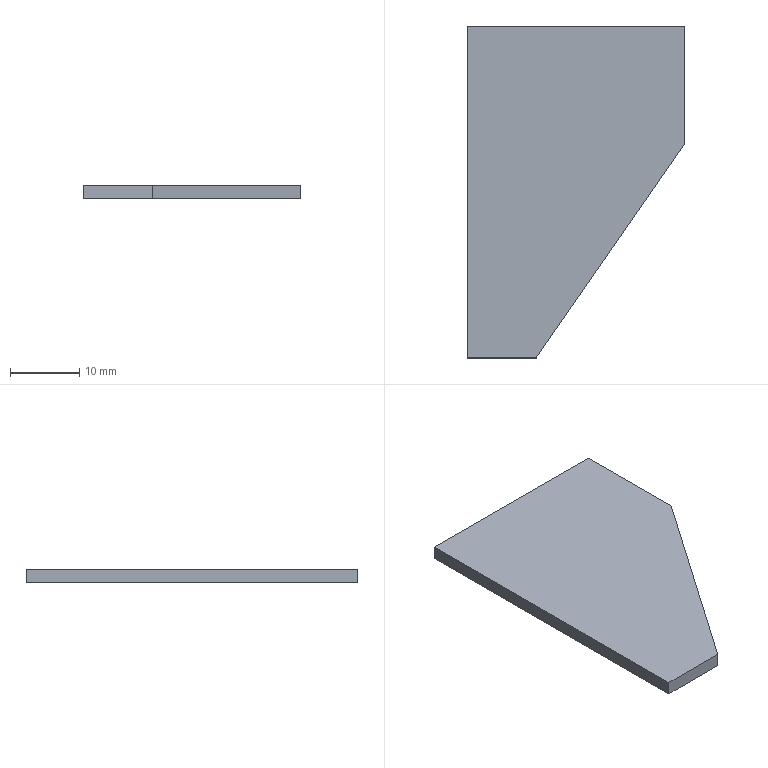Part | 1 solid | 7 faces | box 31.5 x 48 x 2 mm | volume 2357 mm3 | plane 7
STEP:
#1=CARTESIAN_POINT('',(0.,0.,0.));
#2=VERTEX_POINT('',#1);
#3=CARTESIAN_POINT('',(0.,-48.,0.));
#4=VERTEX_POINT('',#3);
#5=CARTESIAN_POINT('',(0.,-48.,0.));
#6=DIRECTION('',(0.,-1.,0.));
#7=VECTOR('',#6,1000.);
#8=LINE('',#5,#7);
#9=EDGE_CURVE('',#2,#4,#8,.T.);
#10=ORIENTED_EDGE('',*,*,#9,.T.);
#11=CARTESIAN_POINT('',(0.,-48.,2.));
#12=VERTEX_POINT('',#11);
#13=CARTESIAN_POINT('',(0.,-48.,2.));
#14=DIRECTION('',(0.,0.,-1.));
#15=VECTOR('',#14,1000.);
#16=LINE('',#13,#15);
#17=EDGE_CURVE('',#12,#4,#16,.T.);
#18=ORIENTED_EDGE('',*,*,#17,.F.);
#19=CARTESIAN_POINT('',(0.,0.,2.));
#20=VERTEX_POINT('',#19);
#21=CARTESIAN_POINT('',(0.,-48.,2.));
#22=DIRECTION('',(0.,-1.,0.));
#23=VECTOR('',#22,1000.);
#24=LINE('',#21,#23);
#25=EDGE_CURVE('',#20,#12,#24,.T.);
#26=ORIENTED_EDGE('',*,*,#25,.F.);
#27=CARTESIAN_POINT('',(0.,0.,2.));
#28=DIRECTION('',(0.,0.,-1.));
#29=VECTOR('',#28,1000.);
#30=LINE('',#27,#29);
#31=EDGE_CURVE('',#20,#2,#30,.T.);
#32=ORIENTED_EDGE('',*,*,#31,.T.);
#33=EDGE_LOOP('',(#10,#18,#26,#32));
#34=FACE_OUTER_BOUND('',#33,.T.);
#35=CARTESIAN_POINT('',(0.,-48.,2.));
#36=DIRECTION('',(1.,0.,0.));
#37=DIRECTION('',(0.,0.,-1.));
#38=AXIS2_PLACEMENT_3D('',#35,#36,#37);
#39=PLANE('',#38);
#40=ADVANCED_FACE('',(#34),#39,.F.);
#41=CARTESIAN_POINT('',(10.,-48.,0.));
#42=VERTEX_POINT('',#41);
#43=CARTESIAN_POINT('',(10.,-48.,0.));
#44=DIRECTION('',(1.,0.,0.));
#45=VECTOR('',#44,1000.);
#46=LINE('',#43,#45);
#47=EDGE_CURVE('',#4,#42,#46,.T.);
#48=ORIENTED_EDGE('',*,*,#47,.T.);
#49=CARTESIAN_POINT('',(10.,-48.,2.));
#50=VERTEX_POINT('',#49);
#51=CARTESIAN_POINT('',(10.,-48.,2.));
#52=DIRECTION('',(0.,0.,-1.));
#53=VECTOR('',#52,1000.);
#54=LINE('',#51,#53);
#55=EDGE_CURVE('',#50,#42,#54,.T.);
#56=ORIENTED_EDGE('',*,*,#55,.F.);
#57=CARTESIAN_POINT('',(10.,-48.,2.));
#58=DIRECTION('',(1.,0.,0.));
#59=VECTOR('',#58,1000.);
#60=LINE('',#57,#59);
#61=EDGE_CURVE('',#12,#50,#60,.T.);
#62=ORIENTED_EDGE('',*,*,#61,.F.);
#63=ORIENTED_EDGE('',*,*,#17,.T.);
#64=EDGE_LOOP('',(#48,#56,#62,#63));
#65=FACE_OUTER_BOUND('',#64,.T.);
#66=CARTESIAN_POINT('',(10.,-48.,2.));
#67=DIRECTION('',(0.,1.,0.));
#68=DIRECTION('',(0.,0.,1.));
#69=AXIS2_PLACEMENT_3D('',#66,#67,#68);
#70=PLANE('',#69);
#71=ADVANCED_FACE('',(#65),#70,.F.);
#72=CARTESIAN_POINT('',(31.5,-17.,0.));
#73=VERTEX_POINT('',#72);
#74=CARTESIAN_POINT('',(31.5,-17.,0.));
#75=DIRECTION('',(0.5699,0.8217,0.));
#76=VECTOR('',#75,1000.);
#77=LINE('',#74,#76);
#78=EDGE_CURVE('',#42,#73,#77,.T.);
#79=ORIENTED_EDGE('',*,*,#78,.T.);
#80=CARTESIAN_POINT('',(31.5,-17.,2.));
#81=VERTEX_POINT('',#80);
#82=CARTESIAN_POINT('',(31.5,-17.,2.));
#83=DIRECTION('',(0.,0.,-1.));
#84=VECTOR('',#83,1000.);
#85=LINE('',#82,#84);
#86=EDGE_CURVE('',#81,#73,#85,.T.);
#87=ORIENTED_EDGE('',*,*,#86,.F.);
#88=CARTESIAN_POINT('',(31.5,-17.,2.));
#89=DIRECTION('',(0.5699,0.8217,0.));
#90=VECTOR('',#89,1000.);
#91=LINE('',#88,#90);
#92=EDGE_CURVE('',#50,#81,#91,.T.);
#93=ORIENTED_EDGE('',*,*,#92,.F.);
#94=ORIENTED_EDGE('',*,*,#55,.T.);
#95=EDGE_LOOP('',(#79,#87,#93,#94));
#96=FACE_OUTER_BOUND('',#95,.T.);
#97=CARTESIAN_POINT('',(31.5,-17.,2.));
#98=DIRECTION('',(-0.8217,0.5699,0.));
#99=DIRECTION('',(-0.5699,-0.8217,0.));
#100=AXIS2_PLACEMENT_3D('',#97,#98,#99);
#101=PLANE('',#100);
#102=ADVANCED_FACE('',(#96),#101,.F.);
#103=CARTESIAN_POINT('',(31.5,0.,0.));
#104=VERTEX_POINT('',#103);
#105=CARTESIAN_POINT('',(31.5,0.,0.));
#106=DIRECTION('',(0.,1.,0.));
#107=VECTOR('',#106,1000.);
#108=LINE('',#105,#107);
#109=EDGE_CURVE('',#73,#104,#108,.T.);
#110=ORIENTED_EDGE('',*,*,#109,.T.);
#111=CARTESIAN_POINT('',(31.5,0.,2.));
#112=VERTEX_POINT('',#111);
#113=CARTESIAN_POINT('',(31.5,0.,2.));
#114=DIRECTION('',(0.,0.,-1.));
#115=VECTOR('',#114,1000.);
#116=LINE('',#113,#115);
#117=EDGE_CURVE('',#112,#104,#116,.T.);
#118=ORIENTED_EDGE('',*,*,#117,.F.);
#119=CARTESIAN_POINT('',(31.5,0.,2.));
#120=DIRECTION('',(0.,1.,0.));
#121=VECTOR('',#120,1000.);
#122=LINE('',#119,#121);
#123=EDGE_CURVE('',#81,#112,#122,.T.);
#124=ORIENTED_EDGE('',*,*,#123,.F.);
#125=ORIENTED_EDGE('',*,*,#86,.T.);
#126=EDGE_LOOP('',(#110,#118,#124,#125));
#127=FACE_OUTER_BOUND('',#126,.T.);
#128=CARTESIAN_POINT('',(31.5,0.,2.));
#129=DIRECTION('',(-1.,0.,0.));
#130=DIRECTION('',(0.,0.,1.));
#131=AXIS2_PLACEMENT_3D('',#128,#129,#130);
#132=PLANE('',#131);
#133=ADVANCED_FACE('',(#127),#132,.F.);
#134=CARTESIAN_POINT('',(0.,0.,0.));
#135=DIRECTION('',(-1.,0.,0.));
#136=VECTOR('',#135,1000.);
#137=LINE('',#134,#136);
#138=EDGE_CURVE('',#104,#2,#137,.T.);
#139=ORIENTED_EDGE('',*,*,#138,.T.);
#140=ORIENTED_EDGE('',*,*,#31,.F.);
#141=CARTESIAN_POINT('',(0.,0.,2.));
#142=DIRECTION('',(-1.,0.,0.));
#143=VECTOR('',#142,1000.);
#144=LINE('',#141,#143);
#145=EDGE_CURVE('',#112,#20,#144,.T.);
#146=ORIENTED_EDGE('',*,*,#145,.F.);
#147=ORIENTED_EDGE('',*,*,#117,.T.);
#148=EDGE_LOOP('',(#139,#140,#146,#147));
#149=FACE_OUTER_BOUND('',#148,.T.);
#150=CARTESIAN_POINT('',(0.,0.,2.));
#151=DIRECTION('',(0.,-1.,0.));
#152=DIRECTION('',(0.,0.,-1.));
#153=AXIS2_PLACEMENT_3D('',#150,#151,#152);
#154=PLANE('',#153);
#155=ADVANCED_FACE('',(#149),#154,.F.);
#156=ORIENTED_EDGE('',*,*,#25,.T.);
#157=ORIENTED_EDGE('',*,*,#61,.T.);
#158=ORIENTED_EDGE('',*,*,#92,.T.);
#159=ORIENTED_EDGE('',*,*,#123,.T.);
#160=ORIENTED_EDGE('',*,*,#145,.T.);
#161=EDGE_LOOP('',(#156,#157,#158,#159,#160));
#162=FACE_OUTER_BOUND('',#161,.T.);
#163=CARTESIAN_POINT('',(0.,0.,2.));
#164=DIRECTION('',(0.,0.,-1.));
#165=DIRECTION('',(-1.,0.,0.));
#166=AXIS2_PLACEMENT_3D('',#163,#164,#165);
#167=PLANE('',#166);
#168=ADVANCED_FACE('',(#162),#167,.F.);
#169=ORIENTED_EDGE('',*,*,#9,.F.);
#170=ORIENTED_EDGE('',*,*,#138,.F.);
#171=ORIENTED_EDGE('',*,*,#109,.F.);
#172=ORIENTED_EDGE('',*,*,#78,.F.);
#173=ORIENTED_EDGE('',*,*,#47,.F.);
#174=EDGE_LOOP('',(#169,#170,#171,#172,#173));
#175=FACE_OUTER_BOUND('',#174,.T.);
#176=CARTESIAN_POINT('',(0.,0.,0.));
#177=DIRECTION('',(0.,0.,-1.));
#178=DIRECTION('',(-1.,0.,0.));
#179=AXIS2_PLACEMENT_3D('',#176,#177,#178);
#180=PLANE('',#179);
#181=ADVANCED_FACE('',(#175),#180,.T.);
#182=CLOSED_SHELL('',(#40,#71,#102,#133,#155,#168,#181));
#183=MANIFOLD_SOLID_BREP('',#182);
#184=CARTESIAN_POINT('',(0.,0.,0.));
#185=DIRECTION('',(0.,0.,1.));
#186=DIRECTION('',(1.,0.,0.));
#187=AXIS2_PLACEMENT_3D('',#184,#185,#186);
#188=(LENGTH_UNIT()NAMED_UNIT(*)SI_UNIT(.MILLI.,.METRE.));
#189=UNCERTAINTY_MEASURE_WITH_UNIT(LENGTH_MEASURE(0.00001),#188,'','');
#190=(NAMED_UNIT(*)PLANE_ANGLE_UNIT()SI_UNIT($,.RADIAN.));
#191=(NAMED_UNIT(*)SI_UNIT($,.STERADIAN.)SOLID_ANGLE_UNIT());
#192=(GEOMETRIC_REPRESENTATION_CONTEXT(3)GLOBAL_UNCERTAINTY_ASSIGNED_CONTEXT((#189))GLOBAL_UNIT_ASSIGNED_CONTEXT((#188,#190,#191))REPRESENTATION_CONTEXT('',''));
#193=ADVANCED_BREP_SHAPE_REPRESENTATION('',(#183,#187),#192);